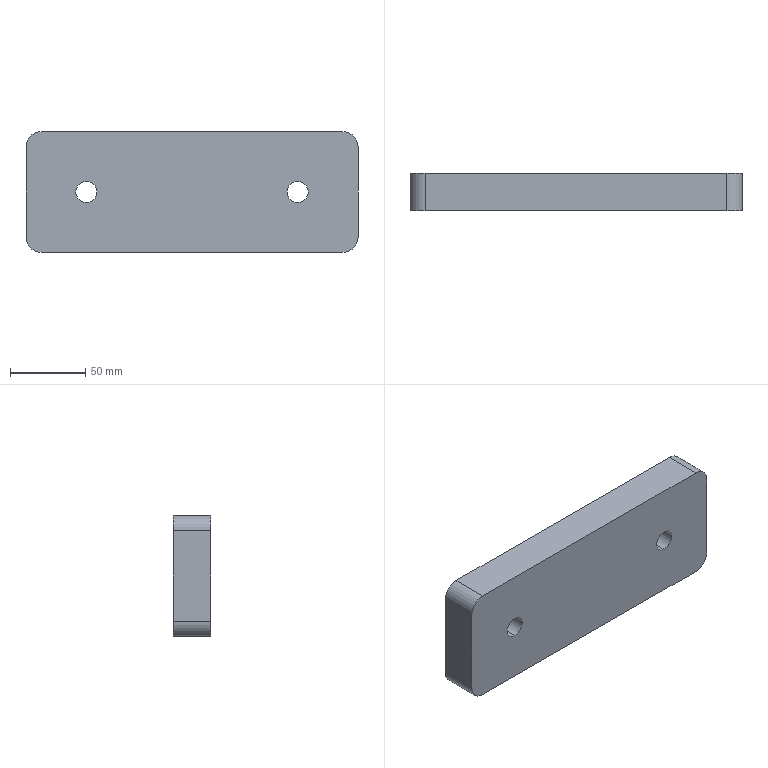Part | SolidWorks | features Fillet 1, FlatPattern 1, HoleWzd 1, LPattern 1, SMBaseFlange 1, SheetMetal 1 | 1 solid | 14 faces | box 220 x 25 x 80 mm | volume 430157 mm3 | cylinder 8 | plane 6 | commonest cylinder face diameters 14 x4 20 x4
STEP:
#1=CARTESIAN_POINT('',(70.,-25.,7.));
#2=VERTEX_POINT('',#1);
#3=CARTESIAN_POINT('',(70.,-25.,-7.));
#4=VERTEX_POINT('',#3);
#5=CARTESIAN_POINT('',(70.,-25.,0.));
#6=DIRECTION('',(0.,-1.,0.));
#7=DIRECTION('',(0.,0.,-1.));
#8=AXIS2_PLACEMENT_3D('',#5,#6,#7);
#9=CIRCLE('',#8,7.);
#10=EDGE_CURVE('',#2,#4,#9,.T.);
#11=ORIENTED_EDGE('',*,*,#10,.T.);
#12=CARTESIAN_POINT('',(70.,0.,-7.));
#13=VERTEX_POINT('',#12);
#14=CARTESIAN_POINT('',(70.,0.,-7.));
#15=DIRECTION('',(0.,1.,0.));
#16=VECTOR('',#15,1000.);
#17=LINE('',#14,#16);
#18=EDGE_CURVE('',#4,#13,#17,.T.);
#19=ORIENTED_EDGE('',*,*,#18,.T.);
#20=CARTESIAN_POINT('',(70.,0.,7.));
#21=VERTEX_POINT('',#20);
#22=CARTESIAN_POINT('',(70.,0.,0.));
#23=DIRECTION('',(0.,1.,0.));
#24=DIRECTION('',(0.,0.,1.));
#25=AXIS2_PLACEMENT_3D('',#22,#23,#24);
#26=CIRCLE('',#25,7.);
#27=EDGE_CURVE('',#13,#21,#26,.T.);
#28=ORIENTED_EDGE('',*,*,#27,.T.);
#29=CARTESIAN_POINT('',(70.,0.,7.));
#30=DIRECTION('',(0.,1.,0.));
#31=VECTOR('',#30,1000.);
#32=LINE('',#29,#31);
#33=EDGE_CURVE('',#2,#21,#32,.T.);
#34=ORIENTED_EDGE('',*,*,#33,.F.);
#35=EDGE_LOOP('',(#11,#19,#28,#34));
#36=FACE_OUTER_BOUND('',#35,.T.);
#37=CARTESIAN_POINT('',(70.,0.,0.));
#38=DIRECTION('',(0.,1.,0.));
#39=DIRECTION('',(0.,0.,1.));
#40=AXIS2_PLACEMENT_3D('',#37,#38,#39);
#41=CYLINDRICAL_SURFACE('',#40,7.);
#42=ADVANCED_FACE('',(#36),#41,.F.);
#43=CARTESIAN_POINT('',(-70.,-25.,7.));
#44=VERTEX_POINT('',#43);
#45=CARTESIAN_POINT('',(-70.,-25.,-7.));
#46=VERTEX_POINT('',#45);
#47=CARTESIAN_POINT('',(-70.,-25.,0.));
#48=DIRECTION('',(0.,-1.,0.));
#49=DIRECTION('',(0.,0.,-1.));
#50=AXIS2_PLACEMENT_3D('',#47,#48,#49);
#51=CIRCLE('',#50,7.);
#52=EDGE_CURVE('',#44,#46,#51,.T.);
#53=ORIENTED_EDGE('',*,*,#52,.T.);
#54=CARTESIAN_POINT('',(-70.,0.,-7.));
#55=VERTEX_POINT('',#54);
#56=CARTESIAN_POINT('',(-70.,0.,-7.));
#57=DIRECTION('',(0.,1.,0.));
#58=VECTOR('',#57,1000.);
#59=LINE('',#56,#58);
#60=EDGE_CURVE('',#46,#55,#59,.T.);
#61=ORIENTED_EDGE('',*,*,#60,.T.);
#62=CARTESIAN_POINT('',(-70.,0.,7.));
#63=VERTEX_POINT('',#62);
#64=CARTESIAN_POINT('',(-70.,0.,0.));
#65=DIRECTION('',(0.,1.,0.));
#66=DIRECTION('',(0.,0.,1.));
#67=AXIS2_PLACEMENT_3D('',#64,#65,#66);
#68=CIRCLE('',#67,7.);
#69=EDGE_CURVE('',#55,#63,#68,.T.);
#70=ORIENTED_EDGE('',*,*,#69,.T.);
#71=CARTESIAN_POINT('',(-70.,0.,7.));
#72=DIRECTION('',(0.,1.,0.));
#73=VECTOR('',#72,1000.);
#74=LINE('',#71,#73);
#75=EDGE_CURVE('',#44,#63,#74,.T.);
#76=ORIENTED_EDGE('',*,*,#75,.F.);
#77=EDGE_LOOP('',(#53,#61,#70,#76));
#78=FACE_OUTER_BOUND('',#77,.T.);
#79=CARTESIAN_POINT('',(-70.,0.,0.));
#80=DIRECTION('',(0.,1.,0.));
#81=DIRECTION('',(0.,0.,1.));
#82=AXIS2_PLACEMENT_3D('',#79,#80,#81);
#83=CYLINDRICAL_SURFACE('',#82,7.);
#84=ADVANCED_FACE('',(#78),#83,.F.);
#85=CARTESIAN_POINT('',(110.,0.,30.));
#86=VERTEX_POINT('',#85);
#87=CARTESIAN_POINT('',(110.,0.,-30.));
#88=VERTEX_POINT('',#87);
#89=CARTESIAN_POINT('',(110.,0.,40.));
#90=DIRECTION('',(0.,0.,-1.));
#91=VECTOR('',#90,1000.);
#92=LINE('',#89,#91);
#93=EDGE_CURVE('',#86,#88,#92,.T.);
#94=ORIENTED_EDGE('',*,*,#93,.F.);
#95=CARTESIAN_POINT('',(110.,-25.,30.));
#96=VERTEX_POINT('',#95);
#97=CARTESIAN_POINT('',(110.,-25.,30.));
#98=DIRECTION('',(0.,-1.,0.));
#99=VECTOR('',#98,1000.);
#100=LINE('',#97,#99);
#101=EDGE_CURVE('',#86,#96,#100,.T.);
#102=ORIENTED_EDGE('',*,*,#101,.T.);
#103=CARTESIAN_POINT('',(110.,-25.,-30.));
#104=VERTEX_POINT('',#103);
#105=CARTESIAN_POINT('',(110.,-25.,40.));
#106=DIRECTION('',(0.,0.,-1.));
#107=VECTOR('',#106,1000.);
#108=LINE('',#105,#107);
#109=EDGE_CURVE('',#96,#104,#108,.T.);
#110=ORIENTED_EDGE('',*,*,#109,.T.);
#111=CARTESIAN_POINT('',(110.,-25.,-30.));
#112=DIRECTION('',(0.,1.,0.));
#113=VECTOR('',#112,1000.);
#114=LINE('',#111,#113);
#115=EDGE_CURVE('',#104,#88,#114,.T.);
#116=ORIENTED_EDGE('',*,*,#115,.T.);
#117=EDGE_LOOP('',(#94,#102,#110,#116));
#118=FACE_OUTER_BOUND('',#117,.T.);
#119=CARTESIAN_POINT('',(110.,-25.,40.));
#120=DIRECTION('',(1.,0.,0.));
#121=DIRECTION('',(0.,0.,-1.));
#122=AXIS2_PLACEMENT_3D('',#119,#120,#121);
#123=PLANE('',#122);
#124=ADVANCED_FACE('',(#118),#123,.T.);
#125=CARTESIAN_POINT('',(-100.,-25.,40.));
#126=VERTEX_POINT('',#125);
#127=CARTESIAN_POINT('',(100.,-25.,40.));
#128=VERTEX_POINT('',#127);
#129=CARTESIAN_POINT('',(-110.,-25.,40.));
#130=DIRECTION('',(1.,0.,0.));
#131=VECTOR('',#130,1000.);
#132=LINE('',#129,#131);
#133=EDGE_CURVE('',#126,#128,#132,.T.);
#134=ORIENTED_EDGE('',*,*,#133,.T.);
#135=CARTESIAN_POINT('',(100.,0.,40.));
#136=VERTEX_POINT('',#135);
#137=CARTESIAN_POINT('',(100.,-25.,40.));
#138=DIRECTION('',(0.,1.,0.));
#139=VECTOR('',#138,1000.);
#140=LINE('',#137,#139);
#141=EDGE_CURVE('',#128,#136,#140,.T.);
#142=ORIENTED_EDGE('',*,*,#141,.T.);
#143=CARTESIAN_POINT('',(-100.,0.,40.));
#144=VERTEX_POINT('',#143);
#145=CARTESIAN_POINT('',(-110.,0.,40.));
#146=DIRECTION('',(1.,0.,0.));
#147=VECTOR('',#146,1000.);
#148=LINE('',#145,#147);
#149=EDGE_CURVE('',#144,#136,#148,.T.);
#150=ORIENTED_EDGE('',*,*,#149,.F.);
#151=CARTESIAN_POINT('',(-100.,-25.,40.));
#152=DIRECTION('',(0.,-1.,0.));
#153=VECTOR('',#152,1000.);
#154=LINE('',#151,#153);
#155=EDGE_CURVE('',#144,#126,#154,.T.);
#156=ORIENTED_EDGE('',*,*,#155,.T.);
#157=EDGE_LOOP('',(#134,#142,#150,#156));
#158=FACE_OUTER_BOUND('',#157,.T.);
#159=CARTESIAN_POINT('',(-110.,-25.,40.));
#160=DIRECTION('',(0.,0.,1.));
#161=DIRECTION('',(1.,0.,0.));
#162=AXIS2_PLACEMENT_3D('',#159,#160,#161);
#163=PLANE('',#162);
#164=ADVANCED_FACE('',(#158),#163,.T.);
#165=CARTESIAN_POINT('',(-110.,-25.,-30.));
#166=VERTEX_POINT('',#165);
#167=CARTESIAN_POINT('',(-110.,-25.,30.));
#168=VERTEX_POINT('',#167);
#169=CARTESIAN_POINT('',(-110.,-25.,40.));
#170=DIRECTION('',(0.,0.,1.));
#171=VECTOR('',#170,1000.);
#172=LINE('',#169,#171);
#173=EDGE_CURVE('',#166,#168,#172,.T.);
#174=ORIENTED_EDGE('',*,*,#173,.T.);
#175=CARTESIAN_POINT('',(-110.,0.,30.));
#176=VERTEX_POINT('',#175);
#177=CARTESIAN_POINT('',(-110.,-25.,30.));
#178=DIRECTION('',(0.,1.,0.));
#179=VECTOR('',#178,1000.);
#180=LINE('',#177,#179);
#181=EDGE_CURVE('',#168,#176,#180,.T.);
#182=ORIENTED_EDGE('',*,*,#181,.T.);
#183=CARTESIAN_POINT('',(-110.,0.,-30.));
#184=VERTEX_POINT('',#183);
#185=CARTESIAN_POINT('',(-110.,0.,40.));
#186=DIRECTION('',(0.,0.,1.));
#187=VECTOR('',#186,1000.);
#188=LINE('',#185,#187);
#189=EDGE_CURVE('',#184,#176,#188,.T.);
#190=ORIENTED_EDGE('',*,*,#189,.F.);
#191=CARTESIAN_POINT('',(-110.,-25.,-30.));
#192=DIRECTION('',(0.,-1.,0.));
#193=VECTOR('',#192,1000.);
#194=LINE('',#191,#193);
#195=EDGE_CURVE('',#184,#166,#194,.T.);
#196=ORIENTED_EDGE('',*,*,#195,.T.);
#197=EDGE_LOOP('',(#174,#182,#190,#196));
#198=FACE_OUTER_BOUND('',#197,.T.);
#199=CARTESIAN_POINT('',(-110.,-25.,40.));
#200=DIRECTION('',(-1.,0.,0.));
#201=DIRECTION('',(0.,0.,1.));
#202=AXIS2_PLACEMENT_3D('',#199,#200,#201);
#203=PLANE('',#202);
#204=ADVANCED_FACE('',(#198),#203,.T.);
#205=CARTESIAN_POINT('',(100.,0.,-40.));
#206=VERTEX_POINT('',#205);
#207=CARTESIAN_POINT('',(-100.,0.,-40.));
#208=VERTEX_POINT('',#207);
#209=CARTESIAN_POINT('',(-110.,0.,-40.));
#210=DIRECTION('',(-1.,0.,0.));
#211=VECTOR('',#210,1000.);
#212=LINE('',#209,#211);
#213=EDGE_CURVE('',#206,#208,#212,.T.);
#214=ORIENTED_EDGE('',*,*,#213,.F.);
#215=CARTESIAN_POINT('',(100.,-25.,-40.));
#216=VERTEX_POINT('',#215);
#217=CARTESIAN_POINT('',(100.,-25.,-40.));
#218=DIRECTION('',(0.,-1.,0.));
#219=VECTOR('',#218,1000.);
#220=LINE('',#217,#219);
#221=EDGE_CURVE('',#206,#216,#220,.T.);
#222=ORIENTED_EDGE('',*,*,#221,.T.);
#223=CARTESIAN_POINT('',(-100.,-25.,-40.));
#224=VERTEX_POINT('',#223);
#225=CARTESIAN_POINT('',(-110.,-25.,-40.));
#226=DIRECTION('',(-1.,0.,0.));
#227=VECTOR('',#226,1000.);
#228=LINE('',#225,#227);
#229=EDGE_CURVE('',#216,#224,#228,.T.);
#230=ORIENTED_EDGE('',*,*,#229,.T.);
#231=CARTESIAN_POINT('',(-100.,-25.,-40.));
#232=DIRECTION('',(0.,1.,0.));
#233=VECTOR('',#232,1000.);
#234=LINE('',#231,#233);
#235=EDGE_CURVE('',#224,#208,#234,.T.);
#236=ORIENTED_EDGE('',*,*,#235,.T.);
#237=EDGE_LOOP('',(#214,#222,#230,#236));
#238=FACE_OUTER_BOUND('',#237,.T.);
#239=CARTESIAN_POINT('',(-110.,-25.,-40.));
#240=DIRECTION('',(0.,0.,-1.));
#241=DIRECTION('',(-1.,0.,0.));
#242=AXIS2_PLACEMENT_3D('',#239,#240,#241);
#243=PLANE('',#242);
#244=ADVANCED_FACE('',(#238),#243,.T.);
#245=ORIENTED_EDGE('',*,*,#10,.F.);
#246=CARTESIAN_POINT('',(70.,-25.,0.));
#247=DIRECTION('',(0.,-1.,0.));
#248=DIRECTION('',(0.,0.,-1.));
#249=AXIS2_PLACEMENT_3D('',#246,#247,#248);
#250=CIRCLE('',#249,7.);
#251=EDGE_CURVE('',#4,#2,#250,.T.);
#252=ORIENTED_EDGE('',*,*,#251,.F.);
#253=EDGE_LOOP('',(#245,#252));
#254=FACE_BOUND('',#253,.T.);
#255=ORIENTED_EDGE('',*,*,#52,.F.);
#256=CARTESIAN_POINT('',(-70.,-25.,0.));
#257=DIRECTION('',(0.,-1.,0.));
#258=DIRECTION('',(0.,0.,-1.));
#259=AXIS2_PLACEMENT_3D('',#256,#257,#258);
#260=CIRCLE('',#259,7.);
#261=EDGE_CURVE('',#46,#44,#260,.T.);
#262=ORIENTED_EDGE('',*,*,#261,.F.);
#263=EDGE_LOOP('',(#255,#262));
#264=FACE_BOUND('',#263,.T.);
#265=ORIENTED_EDGE('',*,*,#109,.F.);
#266=CARTESIAN_POINT('',(100.,-25.,30.));
#267=DIRECTION('',(0.,-1.,0.));
#268=DIRECTION('',(0.,0.,-1.));
#269=AXIS2_PLACEMENT_3D('',#266,#267,#268);
#270=CIRCLE('',#269,10.);
#271=EDGE_CURVE('',#96,#128,#270,.T.);
#272=ORIENTED_EDGE('',*,*,#271,.T.);
#273=ORIENTED_EDGE('',*,*,#133,.F.);
#274=CARTESIAN_POINT('',(-100.,-25.,30.));
#275=DIRECTION('',(0.,-1.,0.));
#276=DIRECTION('',(0.,0.,-1.));
#277=AXIS2_PLACEMENT_3D('',#274,#275,#276);
#278=CIRCLE('',#277,10.);
#279=EDGE_CURVE('',#126,#168,#278,.T.);
#280=ORIENTED_EDGE('',*,*,#279,.T.);
#281=ORIENTED_EDGE('',*,*,#173,.F.);
#282=CARTESIAN_POINT('',(-100.,-25.,-30.));
#283=DIRECTION('',(0.,-1.,0.));
#284=DIRECTION('',(0.,0.,-1.));
#285=AXIS2_PLACEMENT_3D('',#282,#283,#284);
#286=CIRCLE('',#285,10.);
#287=EDGE_CURVE('',#166,#224,#286,.T.);
#288=ORIENTED_EDGE('',*,*,#287,.T.);
#289=ORIENTED_EDGE('',*,*,#229,.F.);
#290=CARTESIAN_POINT('',(100.,-25.,-30.));
#291=DIRECTION('',(0.,-1.,0.));
#292=DIRECTION('',(0.,0.,-1.));
#293=AXIS2_PLACEMENT_3D('',#290,#291,#292);
#294=CIRCLE('',#293,10.);
#295=EDGE_CURVE('',#216,#104,#294,.T.);
#296=ORIENTED_EDGE('',*,*,#295,.T.);
#297=EDGE_LOOP('',(#265,#272,#273,#280,#281,#288,#289,#296));
#298=FACE_OUTER_BOUND('',#297,.T.);
#299=CARTESIAN_POINT('',(0.,-25.,0.));
#300=DIRECTION('',(0.,-1.,0.));
#301=DIRECTION('',(0.,0.,-1.));
#302=AXIS2_PLACEMENT_3D('',#299,#300,#301);
#303=PLANE('',#302);
#304=ADVANCED_FACE('',(#254,#264,#298),#303,.T.);
#305=CARTESIAN_POINT('',(70.,0.,0.));
#306=DIRECTION('',(0.,1.,0.));
#307=DIRECTION('',(0.,0.,1.));
#308=AXIS2_PLACEMENT_3D('',#305,#306,#307);
#309=CIRCLE('',#308,7.);
#310=EDGE_CURVE('',#21,#13,#309,.T.);
#311=ORIENTED_EDGE('',*,*,#310,.F.);
#312=ORIENTED_EDGE('',*,*,#27,.F.);
#313=EDGE_LOOP('',(#311,#312));
#314=FACE_BOUND('',#313,.T.);
#315=CARTESIAN_POINT('',(-70.,0.,0.));
#316=DIRECTION('',(0.,1.,0.));
#317=DIRECTION('',(0.,0.,1.));
#318=AXIS2_PLACEMENT_3D('',#315,#316,#317);
#319=CIRCLE('',#318,7.);
#320=EDGE_CURVE('',#63,#55,#319,.T.);
#321=ORIENTED_EDGE('',*,*,#320,.F.);
#322=ORIENTED_EDGE('',*,*,#69,.F.);
#323=EDGE_LOOP('',(#321,#322));
#324=FACE_BOUND('',#323,.T.);
#325=ORIENTED_EDGE('',*,*,#149,.T.);
#326=CARTESIAN_POINT('',(100.,0.,30.));
#327=DIRECTION('',(0.,1.,0.));
#328=DIRECTION('',(0.,0.,-1.));
#329=AXIS2_PLACEMENT_3D('',#326,#327,#328);
#330=CIRCLE('',#329,10.);
#331=EDGE_CURVE('',#136,#86,#330,.T.);
#332=ORIENTED_EDGE('',*,*,#331,.T.);
#333=ORIENTED_EDGE('',*,*,#93,.T.);
#334=CARTESIAN_POINT('',(100.,0.,-30.));
#335=DIRECTION('',(0.,1.,0.));
#336=DIRECTION('',(0.,0.,-1.));
#337=AXIS2_PLACEMENT_3D('',#334,#335,#336);
#338=CIRCLE('',#337,10.);
#339=EDGE_CURVE('',#88,#206,#338,.T.);
#340=ORIENTED_EDGE('',*,*,#339,.T.);
#341=ORIENTED_EDGE('',*,*,#213,.T.);
#342=CARTESIAN_POINT('',(-100.,0.,-30.));
#343=DIRECTION('',(0.,1.,0.));
#344=DIRECTION('',(0.,0.,-1.));
#345=AXIS2_PLACEMENT_3D('',#342,#343,#344);
#346=CIRCLE('',#345,10.);
#347=EDGE_CURVE('',#208,#184,#346,.T.);
#348=ORIENTED_EDGE('',*,*,#347,.T.);
#349=ORIENTED_EDGE('',*,*,#189,.T.);
#350=CARTESIAN_POINT('',(-100.,0.,30.));
#351=DIRECTION('',(0.,1.,0.));
#352=DIRECTION('',(0.,0.,-1.));
#353=AXIS2_PLACEMENT_3D('',#350,#351,#352);
#354=CIRCLE('',#353,10.);
#355=EDGE_CURVE('',#176,#144,#354,.T.);
#356=ORIENTED_EDGE('',*,*,#355,.T.);
#357=EDGE_LOOP('',(#325,#332,#333,#340,#341,#348,#349,#356));
#358=FACE_OUTER_BOUND('',#357,.T.);
#359=CARTESIAN_POINT('',(0.,0.,0.));
#360=DIRECTION('',(0.,-1.,0.));
#361=DIRECTION('',(0.,0.,-1.));
#362=AXIS2_PLACEMENT_3D('',#359,#360,#361);
#363=PLANE('',#362);
#364=ADVANCED_FACE('',(#314,#324,#358),#363,.F.);
#365=ORIENTED_EDGE('',*,*,#60,.F.);
#366=ORIENTED_EDGE('',*,*,#261,.T.);
#367=ORIENTED_EDGE('',*,*,#75,.T.);
#368=ORIENTED_EDGE('',*,*,#320,.T.);
#369=EDGE_LOOP('',(#365,#366,#367,#368));
#370=FACE_OUTER_BOUND('',#369,.T.);
#371=CARTESIAN_POINT('',(-70.,0.,0.));
#372=DIRECTION('',(0.,1.,0.));
#373=DIRECTION('',(0.,0.,1.));
#374=AXIS2_PLACEMENT_3D('',#371,#372,#373);
#375=CYLINDRICAL_SURFACE('',#374,7.);
#376=ADVANCED_FACE('',(#370),#375,.F.);
#377=ORIENTED_EDGE('',*,*,#18,.F.);
#378=ORIENTED_EDGE('',*,*,#251,.T.);
#379=ORIENTED_EDGE('',*,*,#33,.T.);
#380=ORIENTED_EDGE('',*,*,#310,.T.);
#381=EDGE_LOOP('',(#377,#378,#379,#380));
#382=FACE_OUTER_BOUND('',#381,.T.);
#383=CARTESIAN_POINT('',(70.,0.,0.));
#384=DIRECTION('',(0.,1.,0.));
#385=DIRECTION('',(0.,0.,1.));
#386=AXIS2_PLACEMENT_3D('',#383,#384,#385);
#387=CYLINDRICAL_SURFACE('',#386,7.);
#388=ADVANCED_FACE('',(#382),#387,.F.);
#389=ORIENTED_EDGE('',*,*,#271,.F.);
#390=ORIENTED_EDGE('',*,*,#101,.F.);
#391=ORIENTED_EDGE('',*,*,#331,.F.);
#392=ORIENTED_EDGE('',*,*,#141,.F.);
#393=EDGE_LOOP('',(#389,#390,#391,#392));
#394=FACE_OUTER_BOUND('',#393,.T.);
#395=CARTESIAN_POINT('',(100.,-25.,30.));
#396=DIRECTION('',(0.,1.,0.));
#397=DIRECTION('',(0.,0.,1.));
#398=AXIS2_PLACEMENT_3D('',#395,#396,#397);
#399=CYLINDRICAL_SURFACE('',#398,10.);
#400=ADVANCED_FACE('',(#394),#399,.T.);
#401=ORIENTED_EDGE('',*,*,#295,.F.);
#402=ORIENTED_EDGE('',*,*,#221,.F.);
#403=ORIENTED_EDGE('',*,*,#339,.F.);
#404=ORIENTED_EDGE('',*,*,#115,.F.);
#405=EDGE_LOOP('',(#401,#402,#403,#404));
#406=FACE_OUTER_BOUND('',#405,.T.);
#407=CARTESIAN_POINT('',(100.,-25.,-30.));
#408=DIRECTION('',(0.,1.,0.));
#409=DIRECTION('',(0.,0.,1.));
#410=AXIS2_PLACEMENT_3D('',#407,#408,#409);
#411=CYLINDRICAL_SURFACE('',#410,10.);
#412=ADVANCED_FACE('',(#406),#411,.T.);
#413=ORIENTED_EDGE('',*,*,#279,.F.);
#414=ORIENTED_EDGE('',*,*,#155,.F.);
#415=ORIENTED_EDGE('',*,*,#355,.F.);
#416=ORIENTED_EDGE('',*,*,#181,.F.);
#417=EDGE_LOOP('',(#413,#414,#415,#416));
#418=FACE_OUTER_BOUND('',#417,.T.);
#419=CARTESIAN_POINT('',(-100.,-25.,30.));
#420=DIRECTION('',(0.,1.,0.));
#421=DIRECTION('',(0.,0.,1.));
#422=AXIS2_PLACEMENT_3D('',#419,#420,#421);
#423=CYLINDRICAL_SURFACE('',#422,10.);
#424=ADVANCED_FACE('',(#418),#423,.T.);
#425=ORIENTED_EDGE('',*,*,#287,.F.);
#426=ORIENTED_EDGE('',*,*,#195,.F.);
#427=ORIENTED_EDGE('',*,*,#347,.F.);
#428=ORIENTED_EDGE('',*,*,#235,.F.);
#429=EDGE_LOOP('',(#425,#426,#427,#428));
#430=FACE_OUTER_BOUND('',#429,.T.);
#431=CARTESIAN_POINT('',(-100.,-25.,-30.));
#432=DIRECTION('',(0.,1.,0.));
#433=DIRECTION('',(0.,0.,1.));
#434=AXIS2_PLACEMENT_3D('',#431,#432,#433);
#435=CYLINDRICAL_SURFACE('',#434,10.);
#436=ADVANCED_FACE('',(#430),#435,.T.);
#437=CLOSED_SHELL('',(#42,#84,#124,#164,#204,#244,#304,#364,#376,#388,#400,#412,#424,#436));
#438=MANIFOLD_SOLID_BREP('',#437);
#439=CARTESIAN_POINT('',(0.,0.,0.));
#440=DIRECTION('',(0.,0.,1.));
#441=DIRECTION('',(1.,0.,0.));
#442=AXIS2_PLACEMENT_3D('',#439,#440,#441);
#443=(LENGTH_UNIT()NAMED_UNIT(*)SI_UNIT(.MILLI.,.METRE.));
#444=UNCERTAINTY_MEASURE_WITH_UNIT(LENGTH_MEASURE(0.00001),#443,'','');
#445=(NAMED_UNIT(*)PLANE_ANGLE_UNIT()SI_UNIT($,.RADIAN.));
#446=(NAMED_UNIT(*)SI_UNIT($,.STERADIAN.)SOLID_ANGLE_UNIT());
#447=(GEOMETRIC_REPRESENTATION_CONTEXT(3)GLOBAL_UNCERTAINTY_ASSIGNED_CONTEXT((#444))GLOBAL_UNIT_ASSIGNED_CONTEXT((#443,#445,#446))REPRESENTATION_CONTEXT('',''));
#448=ADVANCED_BREP_SHAPE_REPRESENTATION('',(#438,#442),#447);